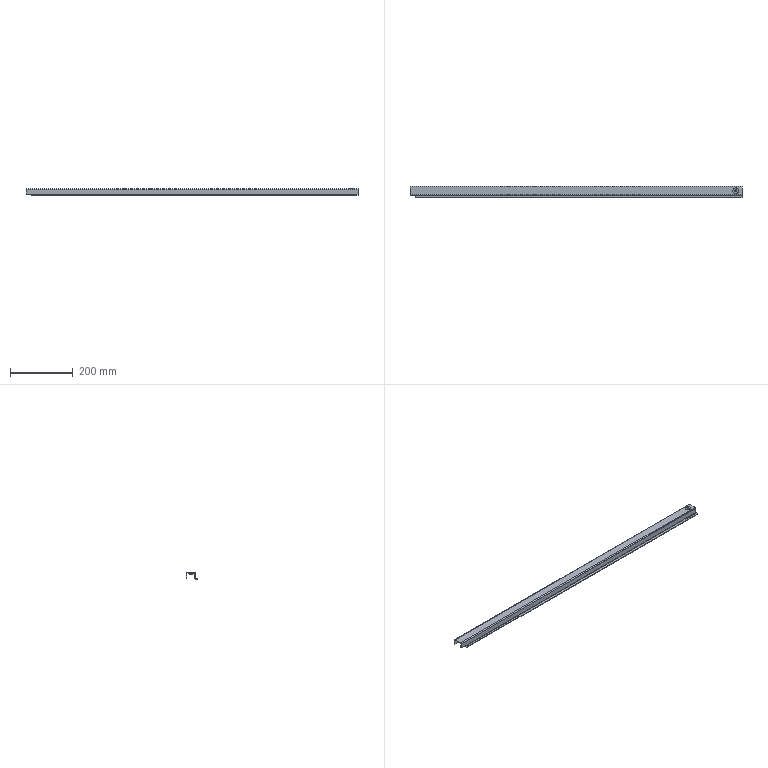Part | SolidWorks | features BaseBody 1 | 1 solid | 48 faces | box 1059 x 38 x 22 mm | volume 155264 mm3 | plane 36 | cylinder 12 | commonest cylinder face diameters 6 x5 2 x3 6.5 x2 18 x2
STEP:
#1=CARTESIAN_POINT('',(500.5,0.,-0.01));
#2=VERTEX_POINT('',#1);
#3=CARTESIAN_POINT('',(500.5,0.,0.));
#4=VERTEX_POINT('',#3);
#5=CARTESIAN_POINT('',(500.5,0.,-0.01));
#6=DIRECTION('',(0.,0.,1.));
#7=VECTOR('',#6,1000.);
#8=LINE('',#5,#7);
#9=EDGE_CURVE('',#2,#4,#8,.T.);
#10=ORIENTED_EDGE('',*,*,#9,.F.);
#11=CARTESIAN_POINT('',(518.5,0.,-0.01));
#12=VERTEX_POINT('',#11);
#13=CARTESIAN_POINT('',(509.5,0.,-0.01));
#14=DIRECTION('',(0.,0.,1.));
#15=DIRECTION('',(1.,0.,0.));
#16=AXIS2_PLACEMENT_3D('',#13,#14,#15);
#17=CIRCLE('',#16,9.);
#18=EDGE_CURVE('',#12,#2,#17,.T.);
#19=ORIENTED_EDGE('',*,*,#18,.F.);
#20=CARTESIAN_POINT('',(518.5,0.,0.));
#21=VERTEX_POINT('',#20);
#22=CARTESIAN_POINT('',(518.5,0.,-0.01));
#23=DIRECTION('',(0.,0.,1.));
#24=VECTOR('',#23,1000.);
#25=LINE('',#22,#24);
#26=EDGE_CURVE('',#12,#21,#25,.T.);
#27=ORIENTED_EDGE('',*,*,#26,.T.);
#28=CARTESIAN_POINT('',(509.5,0.,0.));
#29=DIRECTION('',(0.,0.,1.));
#30=DIRECTION('',(1.,0.,0.));
#31=AXIS2_PLACEMENT_3D('',#28,#29,#30);
#32=CIRCLE('',#31,9.);
#33=EDGE_CURVE('',#21,#4,#32,.T.);
#34=ORIENTED_EDGE('',*,*,#33,.T.);
#35=EDGE_LOOP('',(#10,#19,#27,#34));
#36=FACE_OUTER_BOUND('',#35,.T.);
#37=CARTESIAN_POINT('',(509.5,0.,-0.01));
#38=DIRECTION('',(0.,0.,1.));
#39=DIRECTION('',(1.,0.,0.));
#40=AXIS2_PLACEMENT_3D('',#37,#38,#39);
#41=CYLINDRICAL_SURFACE('',#40,9.);
#42=ADVANCED_FACE('',(#36),#41,.F.);
#43=CARTESIAN_POINT('',(512.75,0.,-0.01));
#44=VERTEX_POINT('',#43);
#45=CARTESIAN_POINT('',(506.25,0.,-0.01));
#46=VERTEX_POINT('',#45);
#47=CARTESIAN_POINT('',(509.5,0.,-0.01));
#48=DIRECTION('',(0.,0.,-1.));
#49=DIRECTION('',(1.,0.,0.));
#50=AXIS2_PLACEMENT_3D('',#47,#48,#49);
#51=CIRCLE('',#50,3.25);
#52=EDGE_CURVE('',#44,#46,#51,.T.);
#53=ORIENTED_EDGE('',*,*,#52,.T.);
#54=CARTESIAN_POINT('',(509.5,0.,-0.01));
#55=DIRECTION('',(0.,0.,-1.));
#56=DIRECTION('',(1.,0.,0.));
#57=AXIS2_PLACEMENT_3D('',#54,#55,#56);
#58=CIRCLE('',#57,3.25);
#59=EDGE_CURVE('',#46,#44,#58,.T.);
#60=ORIENTED_EDGE('',*,*,#59,.T.);
#61=EDGE_LOOP('',(#53,#60));
#62=FACE_BOUND('',#61,.T.);
#63=ORIENTED_EDGE('',*,*,#18,.T.);
#64=CARTESIAN_POINT('',(509.5,0.,-0.01));
#65=DIRECTION('',(0.,0.,1.));
#66=DIRECTION('',(1.,0.,0.));
#67=AXIS2_PLACEMENT_3D('',#64,#65,#66);
#68=CIRCLE('',#67,9.);
#69=EDGE_CURVE('',#2,#12,#68,.T.);
#70=ORIENTED_EDGE('',*,*,#69,.T.);
#71=EDGE_LOOP('',(#63,#70));
#72=FACE_OUTER_BOUND('',#71,.T.);
#73=CARTESIAN_POINT('',(509.5,0.,-0.01));
#74=DIRECTION('',(0.,0.,1.));
#75=DIRECTION('',(1.,0.,0.));
#76=AXIS2_PLACEMENT_3D('',#73,#74,#75);
#77=PLANE('',#76);
#78=ADVANCED_FACE('',(#62,#72),#77,.T.);
#79=CARTESIAN_POINT('',(506.5,0.,-7.));
#80=VERTEX_POINT('',#79);
#81=CARTESIAN_POINT('',(506.5,0.,-2.));
#82=VERTEX_POINT('',#81);
#83=CARTESIAN_POINT('',(506.5,0.,-7.));
#84=DIRECTION('',(0.,0.,1.));
#85=VECTOR('',#84,1000.);
#86=LINE('',#83,#85);
#87=EDGE_CURVE('',#80,#82,#86,.T.);
#88=ORIENTED_EDGE('',*,*,#87,.F.);
#89=CARTESIAN_POINT('',(512.5,0.,-7.));
#90=VERTEX_POINT('',#89);
#91=CARTESIAN_POINT('',(509.5,0.,-7.));
#92=DIRECTION('',(0.,0.,-1.));
#93=DIRECTION('',(-1.,0.,0.));
#94=AXIS2_PLACEMENT_3D('',#91,#92,#93);
#95=CIRCLE('',#94,3.);
#96=EDGE_CURVE('',#80,#90,#95,.T.);
#97=ORIENTED_EDGE('',*,*,#96,.T.);
#98=CARTESIAN_POINT('',(512.5,0.,-2.));
#99=VERTEX_POINT('',#98);
#100=CARTESIAN_POINT('',(512.5,0.,-7.));
#101=DIRECTION('',(0.,0.,1.));
#102=VECTOR('',#101,1000.);
#103=LINE('',#100,#102);
#104=EDGE_CURVE('',#90,#99,#103,.T.);
#105=ORIENTED_EDGE('',*,*,#104,.T.);
#106=CARTESIAN_POINT('',(509.5,0.,-2.));
#107=DIRECTION('',(0.,0.,-1.));
#108=DIRECTION('',(-1.,0.,0.));
#109=AXIS2_PLACEMENT_3D('',#106,#107,#108);
#110=CIRCLE('',#109,3.);
#111=EDGE_CURVE('',#82,#99,#110,.T.);
#112=ORIENTED_EDGE('',*,*,#111,.F.);
#113=EDGE_LOOP('',(#88,#97,#105,#112));
#114=FACE_OUTER_BOUND('',#113,.T.);
#115=CARTESIAN_POINT('',(509.5,0.,-7.));
#116=DIRECTION('',(0.,0.,1.));
#117=DIRECTION('',(1.,0.,0.));
#118=AXIS2_PLACEMENT_3D('',#115,#116,#117);
#119=CYLINDRICAL_SURFACE('',#118,3.);
#120=ADVANCED_FACE('',(#114),#119,.F.);
#121=CARTESIAN_POINT('',(512.387,-5.,-2.));
#122=VERTEX_POINT('',#121);
#123=CARTESIAN_POINT('',(506.613,-5.,-2.));
#124=VERTEX_POINT('',#123);
#125=CARTESIAN_POINT('',(512.387,-5.,-2.));
#126=DIRECTION('',(-1.,0.,0.));
#127=VECTOR('',#126,1000.);
#128=LINE('',#125,#127);
#129=EDGE_CURVE('',#122,#124,#128,.T.);
#130=ORIENTED_EDGE('',*,*,#129,.T.);
#131=CARTESIAN_POINT('',(506.613,-5.,-7.));
#132=VERTEX_POINT('',#131);
#133=CARTESIAN_POINT('',(506.613,-5.,-7.));
#134=DIRECTION('',(0.,0.,1.));
#135=VECTOR('',#134,1000.);
#136=LINE('',#133,#135);
#137=EDGE_CURVE('',#132,#124,#136,.T.);
#138=ORIENTED_EDGE('',*,*,#137,.F.);
#139=CARTESIAN_POINT('',(512.387,-5.,-7.));
#140=VERTEX_POINT('',#139);
#141=CARTESIAN_POINT('',(512.387,-5.,-7.));
#142=DIRECTION('',(-1.,0.,0.));
#143=VECTOR('',#142,1000.);
#144=LINE('',#141,#143);
#145=EDGE_CURVE('',#140,#132,#144,.T.);
#146=ORIENTED_EDGE('',*,*,#145,.F.);
#147=CARTESIAN_POINT('',(512.387,-5.,-7.));
#148=DIRECTION('',(0.,0.,1.));
#149=VECTOR('',#148,1000.);
#150=LINE('',#147,#149);
#151=EDGE_CURVE('',#140,#122,#150,.T.);
#152=ORIENTED_EDGE('',*,*,#151,.T.);
#153=EDGE_LOOP('',(#130,#138,#146,#152));
#154=FACE_OUTER_BOUND('',#153,.T.);
#155=CARTESIAN_POINT('',(512.387,-5.,-7.));
#156=DIRECTION('',(0.,1.,0.));
#157=DIRECTION('',(1.,0.,0.));
#158=AXIS2_PLACEMENT_3D('',#155,#156,#157);
#159=PLANE('',#158);
#160=ADVANCED_FACE('',(#154),#159,.F.);
#161=CARTESIAN_POINT('',(515.274,0.,-2.));
#162=VERTEX_POINT('',#161);
#163=CARTESIAN_POINT('',(515.274,0.,-2.));
#164=DIRECTION('',(-0.5,-0.866,0.));
#165=VECTOR('',#164,1000.);
#166=LINE('',#163,#165);
#167=EDGE_CURVE('',#162,#122,#166,.T.);
#168=ORIENTED_EDGE('',*,*,#167,.T.);
#169=ORIENTED_EDGE('',*,*,#151,.F.);
#170=CARTESIAN_POINT('',(515.274,0.,-7.));
#171=VERTEX_POINT('',#170);
#172=CARTESIAN_POINT('',(515.274,0.,-7.));
#173=DIRECTION('',(-0.5,-0.866,0.));
#174=VECTOR('',#173,1000.);
#175=LINE('',#172,#174);
#176=EDGE_CURVE('',#171,#140,#175,.T.);
#177=ORIENTED_EDGE('',*,*,#176,.F.);
#178=CARTESIAN_POINT('',(515.274,0.,-7.));
#179=DIRECTION('',(0.,0.,1.));
#180=VECTOR('',#179,1000.);
#181=LINE('',#178,#180);
#182=EDGE_CURVE('',#171,#162,#181,.T.);
#183=ORIENTED_EDGE('',*,*,#182,.T.);
#184=EDGE_LOOP('',(#168,#169,#177,#183));
#185=FACE_OUTER_BOUND('',#184,.T.);
#186=CARTESIAN_POINT('',(515.274,0.,-7.));
#187=DIRECTION('',(-0.866,0.5,0.));
#188=DIRECTION('',(0.,0.,1.));
#189=AXIS2_PLACEMENT_3D('',#186,#187,#188);
#190=PLANE('',#189);
#191=ADVANCED_FACE('',(#185),#190,.F.);
#192=CARTESIAN_POINT('',(512.387,5.,-2.));
#193=VERTEX_POINT('',#192);
#194=CARTESIAN_POINT('',(512.387,5.,-2.));
#195=DIRECTION('',(0.5,-0.866,0.));
#196=VECTOR('',#195,1000.);
#197=LINE('',#194,#196);
#198=EDGE_CURVE('',#193,#162,#197,.T.);
#199=ORIENTED_EDGE('',*,*,#198,.T.);
#200=ORIENTED_EDGE('',*,*,#182,.F.);
#201=CARTESIAN_POINT('',(512.387,5.,-7.));
#202=VERTEX_POINT('',#201);
#203=CARTESIAN_POINT('',(512.387,5.,-7.));
#204=DIRECTION('',(0.5,-0.866,0.));
#205=VECTOR('',#204,1000.);
#206=LINE('',#203,#205);
#207=EDGE_CURVE('',#202,#171,#206,.T.);
#208=ORIENTED_EDGE('',*,*,#207,.F.);
#209=CARTESIAN_POINT('',(512.387,5.,-7.));
#210=DIRECTION('',(0.,0.,1.));
#211=VECTOR('',#210,1000.);
#212=LINE('',#209,#211);
#213=EDGE_CURVE('',#202,#193,#212,.T.);
#214=ORIENTED_EDGE('',*,*,#213,.T.);
#215=EDGE_LOOP('',(#199,#200,#208,#214));
#216=FACE_OUTER_BOUND('',#215,.T.);
#217=CARTESIAN_POINT('',(512.387,5.,-7.));
#218=DIRECTION('',(-0.866,-0.5,0.));
#219=DIRECTION('',(-0.5,0.866,0.));
#220=AXIS2_PLACEMENT_3D('',#217,#218,#219);
#221=PLANE('',#220);
#222=ADVANCED_FACE('',(#216),#221,.F.);
#223=CARTESIAN_POINT('',(506.613,5.,-2.));
#224=VERTEX_POINT('',#223);
#225=CARTESIAN_POINT('',(506.613,5.,-2.));
#226=DIRECTION('',(1.,0.,0.));
#227=VECTOR('',#226,1000.);
#228=LINE('',#225,#227);
#229=EDGE_CURVE('',#224,#193,#228,.T.);
#230=ORIENTED_EDGE('',*,*,#229,.T.);
#231=ORIENTED_EDGE('',*,*,#213,.F.);
#232=CARTESIAN_POINT('',(506.613,5.,-7.));
#233=VERTEX_POINT('',#232);
#234=CARTESIAN_POINT('',(506.613,5.,-7.));
#235=DIRECTION('',(1.,0.,0.));
#236=VECTOR('',#235,1000.);
#237=LINE('',#234,#236);
#238=EDGE_CURVE('',#233,#202,#237,.T.);
#239=ORIENTED_EDGE('',*,*,#238,.F.);
#240=CARTESIAN_POINT('',(506.613,5.,-7.));
#241=DIRECTION('',(0.,0.,1.));
#242=VECTOR('',#241,1000.);
#243=LINE('',#240,#242);
#244=EDGE_CURVE('',#233,#224,#243,.T.);
#245=ORIENTED_EDGE('',*,*,#244,.T.);
#246=EDGE_LOOP('',(#230,#231,#239,#245));
#247=FACE_OUTER_BOUND('',#246,.T.);
#248=CARTESIAN_POINT('',(506.613,5.,-7.));
#249=DIRECTION('',(0.,-1.,0.));
#250=DIRECTION('',(0.,0.,-1.));
#251=AXIS2_PLACEMENT_3D('',#248,#249,#250);
#252=PLANE('',#251);
#253=ADVANCED_FACE('',(#247),#252,.F.);
#254=CARTESIAN_POINT('',(503.726,0.,-2.));
#255=VERTEX_POINT('',#254);
#256=CARTESIAN_POINT('',(503.726,0.,-2.));
#257=DIRECTION('',(0.5,0.866,0.));
#258=VECTOR('',#257,1000.);
#259=LINE('',#256,#258);
#260=EDGE_CURVE('',#255,#224,#259,.T.);
#261=ORIENTED_EDGE('',*,*,#260,.T.);
#262=ORIENTED_EDGE('',*,*,#244,.F.);
#263=CARTESIAN_POINT('',(503.726,0.,-7.));
#264=VERTEX_POINT('',#263);
#265=CARTESIAN_POINT('',(503.726,0.,-7.));
#266=DIRECTION('',(0.5,0.866,0.));
#267=VECTOR('',#266,1000.);
#268=LINE('',#265,#267);
#269=EDGE_CURVE('',#264,#233,#268,.T.);
#270=ORIENTED_EDGE('',*,*,#269,.F.);
#271=CARTESIAN_POINT('',(503.726,0.,-7.));
#272=DIRECTION('',(0.,0.,1.));
#273=VECTOR('',#272,1000.);
#274=LINE('',#271,#273);
#275=EDGE_CURVE('',#264,#255,#274,.T.);
#276=ORIENTED_EDGE('',*,*,#275,.T.);
#277=EDGE_LOOP('',(#261,#262,#270,#276));
#278=FACE_OUTER_BOUND('',#277,.T.);
#279=CARTESIAN_POINT('',(503.726,0.,-7.));
#280=DIRECTION('',(0.866,-0.5,0.));
#281=DIRECTION('',(0.,0.,-1.));
#282=AXIS2_PLACEMENT_3D('',#279,#280,#281);
#283=PLANE('',#282);
#284=ADVANCED_FACE('',(#278),#283,.F.);
#285=CARTESIAN_POINT('',(506.613,-5.,-2.));
#286=DIRECTION('',(-0.5,0.866,0.));
#287=VECTOR('',#286,1000.);
#288=LINE('',#285,#287);
#289=EDGE_CURVE('',#124,#255,#288,.T.);
#290=ORIENTED_EDGE('',*,*,#289,.T.);
#291=ORIENTED_EDGE('',*,*,#275,.F.);
#292=CARTESIAN_POINT('',(506.613,-5.,-7.));
#293=DIRECTION('',(-0.5,0.866,0.));
#294=VECTOR('',#293,1000.);
#295=LINE('',#292,#294);
#296=EDGE_CURVE('',#132,#264,#295,.T.);
#297=ORIENTED_EDGE('',*,*,#296,.F.);
#298=ORIENTED_EDGE('',*,*,#137,.T.);
#299=EDGE_LOOP('',(#290,#291,#297,#298));
#300=FACE_OUTER_BOUND('',#299,.T.);
#301=CARTESIAN_POINT('',(506.613,-5.,-7.));
#302=DIRECTION('',(0.866,0.5,0.));
#303=DIRECTION('',(0.,0.,-1.));
#304=AXIS2_PLACEMENT_3D('',#301,#302,#303);
#305=PLANE('',#304);
#306=ADVANCED_FACE('',(#300),#305,.F.);
#307=CARTESIAN_POINT('',(509.5,0.,-7.));
#308=DIRECTION('',(0.,0.,-1.));
#309=DIRECTION('',(-1.,0.,0.));
#310=AXIS2_PLACEMENT_3D('',#307,#308,#309);
#311=CIRCLE('',#310,3.);
#312=EDGE_CURVE('',#90,#80,#311,.T.);
#313=ORIENTED_EDGE('',*,*,#312,.F.);
#314=ORIENTED_EDGE('',*,*,#96,.F.);
#315=EDGE_LOOP('',(#313,#314));
#316=FACE_BOUND('',#315,.T.);
#317=ORIENTED_EDGE('',*,*,#296,.T.);
#318=ORIENTED_EDGE('',*,*,#269,.T.);
#319=ORIENTED_EDGE('',*,*,#238,.T.);
#320=ORIENTED_EDGE('',*,*,#207,.T.);
#321=ORIENTED_EDGE('',*,*,#176,.T.);
#322=ORIENTED_EDGE('',*,*,#145,.T.);
#323=EDGE_LOOP('',(#317,#318,#319,#320,#321,#322));
#324=FACE_OUTER_BOUND('',#323,.T.);
#325=CARTESIAN_POINT('',(0.,0.,-7.));
#326=DIRECTION('',(0.,0.,-1.));
#327=DIRECTION('',(0.,-1.,0.));
#328=AXIS2_PLACEMENT_3D('',#325,#326,#327);
#329=PLANE('',#328);
#330=ADVANCED_FACE('',(#316,#324),#329,.T.);
#331=CARTESIAN_POINT('',(509.5,0.,-2.));
#332=DIRECTION('',(0.,0.,-1.));
#333=DIRECTION('',(-1.,0.,0.));
#334=AXIS2_PLACEMENT_3D('',#331,#332,#333);
#335=CIRCLE('',#334,3.);
#336=EDGE_CURVE('',#99,#82,#335,.T.);
#337=ORIENTED_EDGE('',*,*,#336,.T.);
#338=ORIENTED_EDGE('',*,*,#111,.T.);
#339=EDGE_LOOP('',(#337,#338));
#340=FACE_BOUND('',#339,.T.);
#341=CARTESIAN_POINT('',(512.75,0.,-2.));
#342=VERTEX_POINT('',#341);
#343=CARTESIAN_POINT('',(506.25,0.,-2.));
#344=VERTEX_POINT('',#343);
#345=CARTESIAN_POINT('',(509.5,0.,-2.));
#346=DIRECTION('',(0.,0.,1.));
#347=DIRECTION('',(1.,0.,0.));
#348=AXIS2_PLACEMENT_3D('',#345,#346,#347);
#349=CIRCLE('',#348,3.25);
#350=EDGE_CURVE('',#342,#344,#349,.T.);
#351=ORIENTED_EDGE('',*,*,#350,.T.);
#352=CARTESIAN_POINT('',(509.5,0.,-2.));
#353=DIRECTION('',(0.,0.,1.));
#354=DIRECTION('',(1.,0.,0.));
#355=AXIS2_PLACEMENT_3D('',#352,#353,#354);
#356=CIRCLE('',#355,3.25);
#357=EDGE_CURVE('',#344,#342,#356,.T.);
#358=ORIENTED_EDGE('',*,*,#357,.T.);
#359=EDGE_LOOP('',(#351,#358));
#360=FACE_OUTER_BOUND('',#359,.T.);
#361=CARTESIAN_POINT('',(0.,0.,-2.));
#362=DIRECTION('',(0.,0.,-1.));
#363=DIRECTION('',(0.,-1.,0.));
#364=AXIS2_PLACEMENT_3D('',#361,#362,#363);
#365=PLANE('',#364);
#366=ADVANCED_FACE('',(#340,#360),#365,.F.);
#367=CARTESIAN_POINT('',(-511.5,13.,-18.));
#368=VERTEX_POINT('',#367);
#369=CARTESIAN_POINT('',(-511.5,15.,-18.));
#370=VERTEX_POINT('',#369);
#371=CARTESIAN_POINT('',(-511.5,-23.,-18.));
#372=DIRECTION('',(0.,1.,0.));
#373=VECTOR('',#372,1000.);
#374=LINE('',#371,#373);
#375=EDGE_CURVE('',#368,#370,#374,.T.);
#376=ORIENTED_EDGE('',*,*,#375,.T.);
#377=CARTESIAN_POINT('',(-511.5,15.,-20.));
#378=VERTEX_POINT('',#377);
#379=CARTESIAN_POINT('',(-511.5,15.,-20.));
#380=DIRECTION('',(0.,0.,-1.));
#381=VECTOR('',#380,1000.);
#382=LINE('',#379,#381);
#383=EDGE_CURVE('',#370,#378,#382,.T.);
#384=ORIENTED_EDGE('',*,*,#383,.T.);
#385=CARTESIAN_POINT('',(-511.5,13.,-20.));
#386=VERTEX_POINT('',#385);
#387=CARTESIAN_POINT('',(-511.5,-23.,-20.));
#388=DIRECTION('',(0.,1.,0.));
#389=VECTOR('',#388,1000.);
#390=LINE('',#387,#389);
#391=EDGE_CURVE('',#386,#378,#390,.T.);
#392=ORIENTED_EDGE('',*,*,#391,.F.);
#393=CARTESIAN_POINT('',(-511.5,13.,0.));
#394=DIRECTION('',(0.,0.,-1.));
#395=VECTOR('',#394,1000.);
#396=LINE('',#393,#395);
#397=EDGE_CURVE('',#368,#386,#396,.T.);
#398=ORIENTED_EDGE('',*,*,#397,.F.);
#399=EDGE_LOOP('',(#376,#384,#392,#398));
#400=FACE_OUTER_BOUND('',#399,.T.);
#401=CARTESIAN_POINT('',(-511.5,-23.,-20.));
#402=DIRECTION('',(1.,0.,0.));
#403=DIRECTION('',(0.,1.,0.));
#404=AXIS2_PLACEMENT_3D('',#401,#402,#403);
#405=PLANE('',#404);
#406=ADVANCED_FACE('',(#400),#405,.F.);
#407=CARTESIAN_POINT('',(-529.5,13.,-18.));
#408=VERTEX_POINT('',#407);
#409=CARTESIAN_POINT('',(-529.5,15.,-18.));
#410=VERTEX_POINT('',#409);
#411=CARTESIAN_POINT('',(-529.5,-23.,-18.));
#412=DIRECTION('',(0.,1.,0.));
#413=VECTOR('',#412,1000.);
#414=LINE('',#411,#413);
#415=EDGE_CURVE('',#408,#410,#414,.T.);
#416=ORIENTED_EDGE('',*,*,#415,.T.);
#417=CARTESIAN_POINT('',(-529.5,15.,-18.));
#418=DIRECTION('',(1.,0.,0.));
#419=VECTOR('',#418,1000.);
#420=LINE('',#417,#419);
#421=EDGE_CURVE('',#410,#370,#420,.T.);
#422=ORIENTED_EDGE('',*,*,#421,.T.);
#423=ORIENTED_EDGE('',*,*,#375,.F.);
#424=CARTESIAN_POINT('',(0.,13.,-18.));
#425=DIRECTION('',(1.,0.,0.));
#426=VECTOR('',#425,1000.);
#427=LINE('',#424,#426);
#428=EDGE_CURVE('',#408,#368,#427,.T.);
#429=ORIENTED_EDGE('',*,*,#428,.F.);
#430=EDGE_LOOP('',(#416,#422,#423,#429));
#431=FACE_OUTER_BOUND('',#430,.T.);
#432=CARTESIAN_POINT('',(-529.5,-23.,-18.));
#433=DIRECTION('',(0.,0.,1.));
#434=DIRECTION('',(0.,-1.,0.));
#435=AXIS2_PLACEMENT_3D('',#432,#433,#434);
#436=PLANE('',#435);
#437=ADVANCED_FACE('',(#431),#436,.F.);
#438=CARTESIAN_POINT('',(529.5,-23.,-20.));
#439=VERTEX_POINT('',#438);
#440=CARTESIAN_POINT('',(-511.5,-23.,-20.));
#441=VERTEX_POINT('',#440);
#442=CARTESIAN_POINT('',(-511.5,-23.,-20.));
#443=DIRECTION('',(-1.,0.,0.));
#444=VECTOR('',#443,1000.);
#445=LINE('',#442,#444);
#446=EDGE_CURVE('',#439,#441,#445,.T.);
#447=ORIENTED_EDGE('',*,*,#446,.T.);
#448=CARTESIAN_POINT('',(-511.5,-23.,-22.));
#449=VERTEX_POINT('',#448);
#450=CARTESIAN_POINT('',(-511.5,-23.,-22.));
#451=DIRECTION('',(0.,0.,1.));
#452=VECTOR('',#451,1000.);
#453=LINE('',#450,#452);
#454=EDGE_CURVE('',#449,#441,#453,.T.);
#455=ORIENTED_EDGE('',*,*,#454,.F.);
#456=CARTESIAN_POINT('',(529.5,-23.,-22.));
#457=VERTEX_POINT('',#456);
#458=CARTESIAN_POINT('',(-511.5,-23.,-22.));
#459=DIRECTION('',(-1.,0.,0.));
#460=VECTOR('',#459,1000.);
#461=LINE('',#458,#460);
#462=EDGE_CURVE('',#457,#449,#461,.T.);
#463=ORIENTED_EDGE('',*,*,#462,.F.);
#464=CARTESIAN_POINT('',(529.5,-23.,-22.));
#465=DIRECTION('',(0.,0.,1.));
#466=VECTOR('',#465,1000.);
#467=LINE('',#464,#466);
#468=EDGE_CURVE('',#457,#439,#467,.T.);
#469=ORIENTED_EDGE('',*,*,#468,.T.);
#470=EDGE_LOOP('',(#447,#455,#463,#469));
#471=FACE_OUTER_BOUND('',#470,.T.);
#472=CARTESIAN_POINT('',(-511.5,-23.,-22.));
#473=DIRECTION('',(0.,1.,0.));
#474=DIRECTION('',(0.,0.,-1.));
#475=AXIS2_PLACEMENT_3D('',#472,#473,#474);
#476=PLANE('',#475);
#477=ADVANCED_FACE('',(#471),#476,.F.);
#478=CARTESIAN_POINT('',(529.5,-16.,-20.));
#479=VERTEX_POINT('',#478);
#480=CARTESIAN_POINT('',(529.5,-23.,-20.));
#481=DIRECTION('',(0.,-1.,0.));
#482=VECTOR('',#481,1000.);
#483=LINE('',#480,#482);
#484=EDGE_CURVE('',#479,#439,#483,.T.);
#485=ORIENTED_EDGE('',*,*,#484,.F.);
#486=CARTESIAN_POINT('',(-511.5,-16.,-20.));
#487=VERTEX_POINT('',#486);
#488=CARTESIAN_POINT('',(-511.5,-16.,-20.));
#489=DIRECTION('',(1.,0.,0.));
#490=VECTOR('',#489,1000.);
#491=LINE('',#488,#490);
#492=EDGE_CURVE('',#487,#479,#491,.T.);
#493=ORIENTED_EDGE('',*,*,#492,.F.);
#494=CARTESIAN_POINT('',(-511.5,-15.,-20.));
#495=DIRECTION('',(0.,1.,0.));
#496=VECTOR('',#495,1000.);
#497=LINE('',#494,#496);
#498=EDGE_CURVE('',#441,#487,#497,.T.);
#499=ORIENTED_EDGE('',*,*,#498,.F.);
#500=ORIENTED_EDGE('',*,*,#446,.F.);
#501=EDGE_LOOP('',(#485,#493,#499,#500));
#502=FACE_OUTER_BOUND('',#501,.T.);
#503=CARTESIAN_POINT('',(0.,0.,-20.));
#504=DIRECTION('',(0.,0.,1.));
#505=DIRECTION('',(1.,0.,0.));
#506=AXIS2_PLACEMENT_3D('',#503,#504,#505);
#507=PLANE('',#506);
#508=ADVANCED_FACE('',(#502),#507,.T.);
#509=CARTESIAN_POINT('',(529.5,-16.,-22.));
#510=VERTEX_POINT('',#509);
#511=CARTESIAN_POINT('',(-511.5,-16.,-22.));
#512=VERTEX_POINT('',#511);
#513=CARTESIAN_POINT('',(0.,-16.,-22.));
#514=DIRECTION('',(-1.,0.,0.));
#515=VECTOR('',#514,1000.);
#516=LINE('',#513,#515);
#517=EDGE_CURVE('',#510,#512,#516,.T.);
#518=ORIENTED_EDGE('',*,*,#517,.F.);
#519=CARTESIAN_POINT('',(529.5,-23.,-22.));
#520=DIRECTION('',(0.,-1.,0.));
#521=VECTOR('',#520,1000.);
#522=LINE('',#519,#521);
#523=EDGE_CURVE('',#510,#457,#522,.T.);
#524=ORIENTED_EDGE('',*,*,#523,.T.);
#525=ORIENTED_EDGE('',*,*,#462,.T.);
#526=CARTESIAN_POINT('',(-511.5,-15.,-22.));
#527=DIRECTION('',(0.,1.,0.));
#528=VECTOR('',#527,1000.);
#529=LINE('',#526,#528);
#530=EDGE_CURVE('',#449,#512,#529,.T.);
#531=ORIENTED_EDGE('',*,*,#530,.T.);
#532=EDGE_LOOP('',(#518,#524,#525,#531));
#533=FACE_OUTER_BOUND('',#532,.T.);
#534=CARTESIAN_POINT('',(0.,0.,-22.));
#535=DIRECTION('',(0.,0.,1.));
#536=DIRECTION('',(1.,0.,0.));
#537=AXIS2_PLACEMENT_3D('',#534,#535,#536);
#538=PLANE('',#537);
#539=ADVANCED_FACE('',(#533),#538,.F.);
#540=CARTESIAN_POINT('',(-511.5,-16.,-20.));
#541=DIRECTION('',(0.,0.,-1.));
#542=VECTOR('',#541,1000.);
#543=LINE('',#540,#542);
#544=EDGE_CURVE('',#487,#512,#543,.T.);
#545=ORIENTED_EDGE('',*,*,#544,.T.);
#546=ORIENTED_EDGE('',*,*,#530,.F.);
#547=ORIENTED_EDGE('',*,*,#454,.T.);
#548=ORIENTED_EDGE('',*,*,#498,.T.);
#549=EDGE_LOOP('',(#545,#546,#547,#548));
#550=FACE_OUTER_BOUND('',#549,.T.);
#551=CARTESIAN_POINT('',(-511.5,-15.,-22.));
#552=DIRECTION('',(1.,0.,0.));
#553=DIRECTION('',(0.,0.,-1.));
#554=AXIS2_PLACEMENT_3D('',#551,#552,#553);
#555=PLANE('',#554);
#556=ADVANCED_FACE('',(#550),#555,.F.);
#557=CARTESIAN_POINT('',(529.5,-16.,-20.));
#558=DIRECTION('',(0.,0.,-1.));
#559=VECTOR('',#558,1000.);
#560=LINE('',#557,#559);
#561=EDGE_CURVE('',#479,#510,#560,.T.);
#562=ORIENTED_EDGE('',*,*,#561,.F.);
#563=ORIENTED_EDGE('',*,*,#484,.T.);
#564=ORIENTED_EDGE('',*,*,#468,.F.);
#565=ORIENTED_EDGE('',*,*,#523,.F.);
#566=EDGE_LOOP('',(#562,#563,#564,#565));
#567=FACE_OUTER_BOUND('',#566,.T.);
#568=CARTESIAN_POINT('',(529.5,-23.,-22.));
#569=DIRECTION('',(-1.,0.,0.));
#570=DIRECTION('',(0.,1.,0.));
#571=AXIS2_PLACEMENT_3D('',#568,#569,#570);
#572=PLANE('',#571);
#573=ADVANCED_FACE('',(#567),#572,.F.);
#574=CARTESIAN_POINT('',(529.5,-15.,-19.));
#575=VERTEX_POINT('',#574);
#576=CARTESIAN_POINT('',(-511.5,-15.,-19.));
#577=VERTEX_POINT('',#576);
#578=CARTESIAN_POINT('',(529.5,-15.,-19.));
#579=DIRECTION('',(-1.,0.,0.));
#580=VECTOR('',#579,1000.);
#581=LINE('',#578,#580);
#582=EDGE_CURVE('',#575,#577,#581,.T.);
#583=ORIENTED_EDGE('',*,*,#582,.T.);
#584=CARTESIAN_POINT('',(-511.5,-16.,-19.));
#585=DIRECTION('',(-1.,0.,0.));
#586=DIRECTION('',(0.,0.,-1.));
#587=AXIS2_PLACEMENT_3D('',#584,#585,#586);
#588=CIRCLE('',#587,1.);
#589=EDGE_CURVE('',#577,#487,#588,.T.);
#590=ORIENTED_EDGE('',*,*,#589,.T.);
#591=ORIENTED_EDGE('',*,*,#492,.T.);
#592=CARTESIAN_POINT('',(529.5,-16.,-19.));
#593=DIRECTION('',(1.,0.,0.));
#594=DIRECTION('',(0.,0.,-1.));
#595=AXIS2_PLACEMENT_3D('',#592,#593,#594);
#596=CIRCLE('',#595,1.);
#597=EDGE_CURVE('',#479,#575,#596,.T.);
#598=ORIENTED_EDGE('',*,*,#597,.T.);
#599=EDGE_LOOP('',(#583,#590,#591,#598));
#600=FACE_OUTER_BOUND('',#599,.T.);
#601=CARTESIAN_POINT('',(529.5,-16.,-19.));
#602=DIRECTION('',(1.,0.,0.));
#603=DIRECTION('',(0.,0.,-1.));
#604=AXIS2_PLACEMENT_3D('',#601,#602,#603);
#605=CYLINDRICAL_SURFACE('',#604,1.);
#606=ADVANCED_FACE('',(#600),#605,.F.);
#607=CARTESIAN_POINT('',(529.5,-13.,-19.));
#608=VERTEX_POINT('',#607);
#609=CARTESIAN_POINT('',(-511.5,-13.,-19.));
#610=VERTEX_POINT('',#609);
#611=CARTESIAN_POINT('',(529.5,-13.,-19.));
#612=DIRECTION('',(-1.,0.,0.));
#613=VECTOR('',#612,1000.);
#614=LINE('',#611,#613);
#615=EDGE_CURVE('',#608,#610,#614,.T.);
#616=ORIENTED_EDGE('',*,*,#615,.F.);
#617=CARTESIAN_POINT('',(529.5,-16.,-19.));
#618=DIRECTION('',(1.,0.,0.));
#619=DIRECTION('',(0.,0.,-1.));
#620=AXIS2_PLACEMENT_3D('',#617,#618,#619);
#621=CIRCLE('',#620,3.);
#622=EDGE_CURVE('',#510,#608,#621,.T.);
#623=ORIENTED_EDGE('',*,*,#622,.F.);
#624=ORIENTED_EDGE('',*,*,#517,.T.);
#625=CARTESIAN_POINT('',(-511.5,-16.,-19.));
#626=DIRECTION('',(-1.,0.,0.));
#627=DIRECTION('',(0.,0.,-1.));
#628=AXIS2_PLACEMENT_3D('',#625,#626,#627);
#629=CIRCLE('',#628,3.);
#630=EDGE_CURVE('',#610,#512,#629,.T.);
#631=ORIENTED_EDGE('',*,*,#630,.F.);
#632=EDGE_LOOP('',(#616,#623,#624,#631));
#633=FACE_OUTER_BOUND('',#632,.T.);
#634=CARTESIAN_POINT('',(529.5,-16.,-19.));
#635=DIRECTION('',(1.,0.,0.));
#636=DIRECTION('',(0.,0.,-1.));
#637=AXIS2_PLACEMENT_3D('',#634,#635,#636);
#638=CYLINDRICAL_SURFACE('',#637,3.);
#639=ADVANCED_FACE('',(#633),#638,.T.);
#640=ORIENTED_EDGE('',*,*,#597,.F.);
#641=ORIENTED_EDGE('',*,*,#561,.T.);
#642=ORIENTED_EDGE('',*,*,#622,.T.);
#643=CARTESIAN_POINT('',(529.5,-15.,-19.));
#644=DIRECTION('',(0.,1.,0.));
#645=VECTOR('',#644,1000.);
#646=LINE('',#643,#645);
#647=EDGE_CURVE('',#575,#608,#646,.T.);
#648=ORIENTED_EDGE('',*,*,#647,.F.);
#649=EDGE_LOOP('',(#640,#641,#642,#648));
#650=FACE_OUTER_BOUND('',#649,.T.);
#651=CARTESIAN_POINT('',(529.5,-16.,-19.));
#652=DIRECTION('',(-1.,0.,0.));
#653=DIRECTION('',(0.,0.,1.));
#654=AXIS2_PLACEMENT_3D('',#651,#652,#653);
#655=PLANE('',#654);
#656=ADVANCED_FACE('',(#650),#655,.F.);
#657=CARTESIAN_POINT('',(-511.5,-13.,-18.));
#658=VERTEX_POINT('',#657);
#659=CARTESIAN_POINT('',(-529.5,-13.,-18.));
#660=VERTEX_POINT('',#659);
#661=CARTESIAN_POINT('',(0.,-13.,-18.));
#662=DIRECTION('',(-1.,0.,0.));
#663=VECTOR('',#662,1000.);
#664=LINE('',#661,#663);
#665=EDGE_CURVE('',#658,#660,#664,.T.);
#666=ORIENTED_EDGE('',*,*,#665,.F.);
#667=CARTESIAN_POINT('',(-511.5,-15.,-18.));
#668=VERTEX_POINT('',#667);
#669=CARTESIAN_POINT('',(-511.5,-15.,-18.));
#670=DIRECTION('',(0.,1.,0.));
#671=VECTOR('',#670,1000.);
#672=LINE('',#669,#671);
#673=EDGE_CURVE('',#668,#658,#672,.T.);
#674=ORIENTED_EDGE('',*,*,#673,.F.);
#675=CARTESIAN_POINT('',(-529.5,-15.,-18.));
#676=VERTEX_POINT('',#675);
#677=CARTESIAN_POINT('',(-511.5,-15.,-18.));
#678=DIRECTION('',(-1.,0.,0.));
#679=VECTOR('',#678,1000.);
#680=LINE('',#677,#679);
#681=EDGE_CURVE('',#668,#676,#680,.T.);
#682=ORIENTED_EDGE('',*,*,#681,.T.);
#683=CARTESIAN_POINT('',(-529.5,-23.,-18.));
#684=DIRECTION('',(0.,1.,0.));
#685=VECTOR('',#684,1000.);
#686=LINE('',#683,#685);
#687=EDGE_CURVE('',#676,#660,#686,.T.);
#688=ORIENTED_EDGE('',*,*,#687,.T.);
#689=EDGE_LOOP('',(#666,#674,#682,#688));
#690=FACE_OUTER_BOUND('',#689,.T.);
#691=CARTESIAN_POINT('',(-511.5,-15.,-18.));
#692=DIRECTION('',(0.,0.,-1.));
#693=DIRECTION('',(0.,-1.,0.));
#694=AXIS2_PLACEMENT_3D('',#691,#692,#693);
#695=PLANE('',#694);
#696=ADVANCED_FACE('',(#690),#695,.T.);
#697=CARTESIAN_POINT('',(-511.5,-13.,0.));
#698=DIRECTION('',(0.,0.,1.));
#699=VECTOR('',#698,1000.);
#700=LINE('',#697,#699);
#701=EDGE_CURVE('',#610,#658,#700,.T.);
#702=ORIENTED_EDGE('',*,*,#701,.F.);
#703=ORIENTED_EDGE('',*,*,#630,.T.);
#704=ORIENTED_EDGE('',*,*,#544,.F.);
#705=ORIENTED_EDGE('',*,*,#589,.F.);
#706=CARTESIAN_POINT('',(-511.5,-15.,-19.));
#707=DIRECTION('',(0.,0.,1.));
#708=VECTOR('',#707,1000.);
#709=LINE('',#706,#708);
#710=EDGE_CURVE('',#577,#668,#709,.T.);
#711=ORIENTED_EDGE('',*,*,#710,.T.);
#712=ORIENTED_EDGE('',*,*,#673,.T.);
#713=EDGE_LOOP('',(#702,#703,#704,#705,#711,#712));
#714=FACE_OUTER_BOUND('',#713,.T.);
#715=CARTESIAN_POINT('',(-511.5,-15.,-19.));
#716=DIRECTION('',(-1.,0.,0.));
#717=DIRECTION('',(0.,1.,0.));
#718=AXIS2_PLACEMENT_3D('',#715,#716,#717);
#719=PLANE('',#718);
#720=ADVANCED_FACE('',(#714),#719,.T.);
#721=ORIENTED_EDGE('',*,*,#687,.F.);
#722=CARTESIAN_POINT('',(-529.5,-15.,-3.));
#723=VERTEX_POINT('',#722);
#724=CARTESIAN_POINT('',(-529.5,-15.,-20.));
#725=DIRECTION('',(0.,0.,1.));
#726=VECTOR('',#725,1000.);
#727=LINE('',#724,#726);
#728=EDGE_CURVE('',#676,#723,#727,.T.);
#729=ORIENTED_EDGE('',*,*,#728,.T.);
#730=CARTESIAN_POINT('',(-529.5,-13.,-3.));
#731=VERTEX_POINT('',#730);
#732=CARTESIAN_POINT('',(-529.5,-13.,-3.));
#733=DIRECTION('',(0.,-1.,0.));
#734=VECTOR('',#733,1000.);
#735=LINE('',#732,#734);
#736=EDGE_CURVE('',#731,#723,#735,.T.);
#737=ORIENTED_EDGE('',*,*,#736,.F.);
#738=CARTESIAN_POINT('',(-529.5,-13.,0.));
#739=DIRECTION('',(0.,0.,1.));
#740=VECTOR('',#739,1000.);
#741=LINE('',#738,#740);
#742=EDGE_CURVE('',#660,#731,#741,.T.);
#743=ORIENTED_EDGE('',*,*,#742,.F.);
#744=EDGE_LOOP('',(#721,#729,#737,#743));
#745=FACE_OUTER_BOUND('',#744,.T.);
#746=CARTESIAN_POINT('',(-529.5,-15.,-20.));
#747=DIRECTION('',(-1.,0.,0.));
#748=DIRECTION('',(0.,0.,1.));
#749=AXIS2_PLACEMENT_3D('',#746,#747,#748);
#750=PLANE('',#749);
#751=ADVANCED_FACE('',(#745),#750,.T.);
#752=CARTESIAN_POINT('',(-529.5,-12.,-2.));
#753=VERTEX_POINT('',#752);
#754=CARTESIAN_POINT('',(529.5,-12.,-2.));
#755=VERTEX_POINT('',#754);
#756=CARTESIAN_POINT('',(-529.5,-12.,-2.));
#757=DIRECTION('',(1.,0.,0.));
#758=VECTOR('',#757,1000.);
#759=LINE('',#756,#758);
#760=EDGE_CURVE('',#753,#755,#759,.T.);
#761=ORIENTED_EDGE('',*,*,#760,.T.);
#762=CARTESIAN_POINT('',(529.5,-13.,-3.));
#763=VERTEX_POINT('',#762);
#764=CARTESIAN_POINT('',(529.5,-12.,-3.));
#765=DIRECTION('',(1.,0.,0.));
#766=DIRECTION('',(0.,0.,1.));
#767=AXIS2_PLACEMENT_3D('',#764,#765,#766);
#768=CIRCLE('',#767,1.);
#769=EDGE_CURVE('',#755,#763,#768,.T.);
#770=ORIENTED_EDGE('',*,*,#769,.T.);
#771=CARTESIAN_POINT('',(529.5,-13.,-3.));
#772=DIRECTION('',(-1.,0.,0.));
#773=VECTOR('',#772,1000.);
#774=LINE('',#771,#773);
#775=EDGE_CURVE('',#763,#731,#774,.T.);
#776=ORIENTED_EDGE('',*,*,#775,.T.);
#777=CARTESIAN_POINT('',(-529.5,-12.,-3.));
#778=DIRECTION('',(-1.,0.,0.));
#779=DIRECTION('',(0.,0.,1.));
#780=AXIS2_PLACEMENT_3D('',#777,#778,#779);
#781=CIRCLE('',#780,1.);
#782=EDGE_CURVE('',#731,#753,#781,.T.);
#783=ORIENTED_EDGE('',*,*,#782,.T.);
#784=EDGE_LOOP('',(#761,#770,#776,#783));
#785=FACE_OUTER_BOUND('',#784,.T.);
#786=CARTESIAN_POINT('',(-529.5,-12.,-3.));
#787=DIRECTION('',(-1.,0.,0.));
#788=DIRECTION('',(0.,-1.,0.));
#789=AXIS2_PLACEMENT_3D('',#786,#787,#788);
#790=CYLINDRICAL_SURFACE('',#789,1.);
#791=ADVANCED_FACE('',(#785),#790,.F.);
#792=CARTESIAN_POINT('',(-529.5,-12.,0.));
#793=VERTEX_POINT('',#792);
#794=CARTESIAN_POINT('',(529.5,-12.,0.));
#795=VERTEX_POINT('',#794);
#796=CARTESIAN_POINT('',(-529.5,-12.,0.));
#797=DIRECTION('',(1.,0.,0.));
#798=VECTOR('',#797,1000.);
#799=LINE('',#796,#798);
#800=EDGE_CURVE('',#793,#795,#799,.T.);
#801=ORIENTED_EDGE('',*,*,#800,.F.);
#802=CARTESIAN_POINT('',(-529.5,-12.,-3.));
#803=DIRECTION('',(-1.,0.,0.));
#804=DIRECTION('',(0.,0.,1.));
#805=AXIS2_PLACEMENT_3D('',#802,#803,#804);
#806=CIRCLE('',#805,3.);
#807=EDGE_CURVE('',#723,#793,#806,.T.);
#808=ORIENTED_EDGE('',*,*,#807,.F.);
#809=CARTESIAN_POINT('',(529.5,-15.,-3.));
#810=VERTEX_POINT('',#809);
#811=CARTESIAN_POINT('',(529.5,-15.,-3.));
#812=DIRECTION('',(1.,0.,0.));
#813=VECTOR('',#812,1000.);
#814=LINE('',#811,#813);
#815=EDGE_CURVE('',#723,#810,#814,.T.);
#816=ORIENTED_EDGE('',*,*,#815,.T.);
#817=CARTESIAN_POINT('',(529.5,-12.,-3.));
#818=DIRECTION('',(1.,0.,0.));
#819=DIRECTION('',(0.,0.,1.));
#820=AXIS2_PLACEMENT_3D('',#817,#818,#819);
#821=CIRCLE('',#820,3.);
#822=EDGE_CURVE('',#795,#810,#821,.T.);
#823=ORIENTED_EDGE('',*,*,#822,.F.);
#824=EDGE_LOOP('',(#801,#808,#816,#823));
#825=FACE_OUTER_BOUND('',#824,.T.);
#826=CARTESIAN_POINT('',(-529.5,-12.,-3.));
#827=DIRECTION('',(-1.,0.,0.));
#828=DIRECTION('',(0.,-1.,0.));
#829=AXIS2_PLACEMENT_3D('',#826,#827,#828);
#830=CYLINDRICAL_SURFACE('',#829,3.);
#831=ADVANCED_FACE('',(#825),#830,.T.);
#832=ORIENTED_EDGE('',*,*,#782,.F.);
#833=ORIENTED_EDGE('',*,*,#736,.T.);
#834=ORIENTED_EDGE('',*,*,#807,.T.);
#835=CARTESIAN_POINT('',(-529.5,-12.,-2.));
#836=DIRECTION('',(0.,0.,1.));
#837=VECTOR('',#836,1000.);
#838=LINE('',#835,#837);
#839=EDGE_CURVE('',#753,#793,#838,.T.);
#840=ORIENTED_EDGE('',*,*,#839,.F.);
#841=EDGE_LOOP('',(#832,#833,#834,#840));
#842=FACE_OUTER_BOUND('',#841,.T.);
#843=CARTESIAN_POINT('',(-529.5,-12.,-3.));
#844=DIRECTION('',(1.,0.,0.));
#845=DIRECTION('',(0.,1.,0.));
#846=AXIS2_PLACEMENT_3D('',#843,#844,#845);
#847=PLANE('',#846);
#848=ADVANCED_FACE('',(#842),#847,.F.);
#849=CARTESIAN_POINT('',(529.5,-15.,-3.));
#850=DIRECTION('',(0.,-1.,0.));
#851=VECTOR('',#850,1000.);
#852=LINE('',#849,#851);
#853=EDGE_CURVE('',#763,#810,#852,.T.);
#854=ORIENTED_EDGE('',*,*,#853,.F.);
#855=ORIENTED_EDGE('',*,*,#769,.F.);
#856=CARTESIAN_POINT('',(529.5,-12.,-2.));
#857=DIRECTION('',(0.,0.,1.));
#858=VECTOR('',#857,1000.);
#859=LINE('',#856,#858);
#860=EDGE_CURVE('',#755,#795,#859,.T.);
#861=ORIENTED_EDGE('',*,*,#860,.T.);
#862=ORIENTED_EDGE('',*,*,#822,.T.);
#863=EDGE_LOOP('',(#854,#855,#861,#862));
#864=FACE_OUTER_BOUND('',#863,.T.);
#865=CARTESIAN_POINT('',(529.5,-12.,-3.));
#866=DIRECTION('',(1.,0.,0.));
#867=DIRECTION('',(0.,1.,0.));
#868=AXIS2_PLACEMENT_3D('',#865,#866,#867);
#869=PLANE('',#868);
#870=ADVANCED_FACE('',(#864),#869,.T.);
#871=ORIENTED_EDGE('',*,*,#391,.T.);
#872=CARTESIAN_POINT('',(529.5,15.,-20.));
#873=VERTEX_POINT('',#872);
#874=CARTESIAN_POINT('',(529.5,15.,-20.));
#875=DIRECTION('',(1.,0.,0.));
#876=VECTOR('',#875,1000.);
#877=LINE('',#874,#876);
#878=EDGE_CURVE('',#378,#873,#877,.T.);
#879=ORIENTED_EDGE('',*,*,#878,.T.);
#880=CARTESIAN_POINT('',(529.5,13.,-20.));
#881=VERTEX_POINT('',#880);
#882=CARTESIAN_POINT('',(529.5,15.,-20.));
#883=DIRECTION('',(0.,-1.,0.));
#884=VECTOR('',#883,1000.);
#885=LINE('',#882,#884);
#886=EDGE_CURVE('',#873,#881,#885,.T.);
#887=ORIENTED_EDGE('',*,*,#886,.T.);
#888=CARTESIAN_POINT('',(0.,13.,-20.));
#889=DIRECTION('',(1.,0.,0.));
#890=VECTOR('',#889,1000.);
#891=LINE('',#888,#890);
#892=EDGE_CURVE('',#386,#881,#891,.T.);
#893=ORIENTED_EDGE('',*,*,#892,.F.);
#894=EDGE_LOOP('',(#871,#879,#887,#893));
#895=FACE_OUTER_BOUND('',#894,.T.);
#896=CARTESIAN_POINT('',(529.5,15.,-20.));
#897=DIRECTION('',(0.,0.,-1.));
#898=DIRECTION('',(-1.,0.,0.));
#899=AXIS2_PLACEMENT_3D('',#896,#897,#898);
#900=PLANE('',#899);
#901=ADVANCED_FACE('',(#895),#900,.T.);
#902=ORIENTED_EDGE('',*,*,#428,.T.);
#903=ORIENTED_EDGE('',*,*,#397,.T.);
#904=ORIENTED_EDGE('',*,*,#892,.T.);
#905=CARTESIAN_POINT('',(529.5,13.,-3.));
#906=VERTEX_POINT('',#905);
#907=CARTESIAN_POINT('',(529.5,13.,0.));
#908=DIRECTION('',(0.,0.,1.));
#909=VECTOR('',#908,1000.);
#910=LINE('',#907,#909);
#911=EDGE_CURVE('',#881,#906,#910,.T.);
#912=ORIENTED_EDGE('',*,*,#911,.T.);
#913=CARTESIAN_POINT('',(-529.5,13.,-3.));
#914=VERTEX_POINT('',#913);
#915=CARTESIAN_POINT('',(-529.5,13.,-3.));
#916=DIRECTION('',(1.,0.,0.));
#917=VECTOR('',#916,1000.);
#918=LINE('',#915,#917);
#919=EDGE_CURVE('',#914,#906,#918,.T.);
#920=ORIENTED_EDGE('',*,*,#919,.F.);
#921=CARTESIAN_POINT('',(-529.5,13.,0.));
#922=DIRECTION('',(0.,0.,-1.));
#923=VECTOR('',#922,1000.);
#924=LINE('',#921,#923);
#925=EDGE_CURVE('',#914,#408,#924,.T.);
#926=ORIENTED_EDGE('',*,*,#925,.T.);
#927=EDGE_LOOP('',(#902,#903,#904,#912,#920,#926));
#928=FACE_OUTER_BOUND('',#927,.T.);
#929=CARTESIAN_POINT('',(0.,13.,0.));
#930=DIRECTION('',(0.,1.,0.));
#931=DIRECTION('',(0.,0.,-1.));
#932=AXIS2_PLACEMENT_3D('',#929,#930,#931);
#933=PLANE('',#932);
#934=ADVANCED_FACE('',(#928),#933,.F.);
#935=ORIENTED_EDGE('',*,*,#383,.F.);
#936=ORIENTED_EDGE('',*,*,#421,.F.);
#937=CARTESIAN_POINT('',(-529.5,15.,-3.));
#938=VERTEX_POINT('',#937);
#939=CARTESIAN_POINT('',(-529.5,15.,-20.));
#940=DIRECTION('',(0.,0.,-1.));
#941=VECTOR('',#940,1000.);
#942=LINE('',#939,#941);
#943=EDGE_CURVE('',#938,#410,#942,.T.);
#944=ORIENTED_EDGE('',*,*,#943,.F.);
#945=CARTESIAN_POINT('',(529.5,15.,-3.));
#946=VERTEX_POINT('',#945);
#947=CARTESIAN_POINT('',(0.,15.,-3.));
#948=DIRECTION('',(1.,0.,0.));
#949=VECTOR('',#948,1000.);
#950=LINE('',#947,#949);
#951=EDGE_CURVE('',#938,#946,#950,.T.);
#952=ORIENTED_EDGE('',*,*,#951,.T.);
#953=CARTESIAN_POINT('',(529.5,15.,-2.));
#954=DIRECTION('',(0.,0.,1.));
#955=VECTOR('',#954,1000.);
#956=LINE('',#953,#955);
#957=EDGE_CURVE('',#873,#946,#956,.T.);
#958=ORIENTED_EDGE('',*,*,#957,.F.);
#959=ORIENTED_EDGE('',*,*,#878,.F.);
#960=EDGE_LOOP('',(#935,#936,#944,#952,#958,#959));
#961=FACE_OUTER_BOUND('',#960,.T.);
#962=CARTESIAN_POINT('',(0.,15.,0.));
#963=DIRECTION('',(0.,1.,0.));
#964=DIRECTION('',(0.,0.,-1.));
#965=AXIS2_PLACEMENT_3D('',#962,#963,#964);
#966=PLANE('',#965);
#967=ADVANCED_FACE('',(#961),#966,.T.);
#968=ORIENTED_EDGE('',*,*,#415,.F.);
#969=ORIENTED_EDGE('',*,*,#925,.F.);
#970=CARTESIAN_POINT('',(-529.5,15.,-3.));
#971=DIRECTION('',(0.,1.,0.));
#972=VECTOR('',#971,1000.);
#973=LINE('',#970,#972);
#974=EDGE_CURVE('',#914,#938,#973,.T.);
#975=ORIENTED_EDGE('',*,*,#974,.T.);
#976=ORIENTED_EDGE('',*,*,#943,.T.);
#977=EDGE_LOOP('',(#968,#969,#975,#976));
#978=FACE_OUTER_BOUND('',#977,.T.);
#979=CARTESIAN_POINT('',(-529.5,15.,-20.));
#980=DIRECTION('',(-1.,0.,0.));
#981=DIRECTION('',(0.,0.,1.));
#982=AXIS2_PLACEMENT_3D('',#979,#980,#981);
#983=PLANE('',#982);
#984=ADVANCED_FACE('',(#978),#983,.T.);
#985=ORIENTED_EDGE('',*,*,#957,.T.);
#986=CARTESIAN_POINT('',(529.5,13.,-3.));
#987=DIRECTION('',(0.,1.,0.));
#988=VECTOR('',#987,1000.);
#989=LINE('',#986,#988);
#990=EDGE_CURVE('',#906,#946,#989,.T.);
#991=ORIENTED_EDGE('',*,*,#990,.F.);
#992=ORIENTED_EDGE('',*,*,#911,.F.);
#993=ORIENTED_EDGE('',*,*,#886,.F.);
#994=EDGE_LOOP('',(#985,#991,#992,#993));
#995=FACE_OUTER_BOUND('',#994,.T.);
#996=CARTESIAN_POINT('',(529.5,15.,-2.));
#997=DIRECTION('',(1.,0.,0.));
#998=DIRECTION('',(0.,1.,0.));
#999=AXIS2_PLACEMENT_3D('',#996,#997,#998);
#1000=PLANE('',#999);
#1001=ADVANCED_FACE('',(#995),#1000,.T.);
#1002=CARTESIAN_POINT('',(529.5,12.,-2.));
#1003=VERTEX_POINT('',#1002);
#1004=CARTESIAN_POINT('',(-529.5,12.,-2.));
#1005=VERTEX_POINT('',#1004);
#1006=CARTESIAN_POINT('',(529.5,12.,-2.));
#1007=DIRECTION('',(-1.,0.,0.));
#1008=VECTOR('',#1007,1000.);
#1009=LINE('',#1006,#1008);
#1010=EDGE_CURVE('',#1003,#1005,#1009,.T.);
#1011=ORIENTED_EDGE('',*,*,#1010,.T.);
#1012=CARTESIAN_POINT('',(-529.5,12.,-3.));
#1013=DIRECTION('',(-1.,0.,0.));
#1014=DIRECTION('',(0.,0.,-1.));
#1015=AXIS2_PLACEMENT_3D('',#1012,#1013,#1014);
#1016=CIRCLE('',#1015,1.);
#1017=EDGE_CURVE('',#1005,#914,#1016,.T.);
#1018=ORIENTED_EDGE('',*,*,#1017,.T.);
#1019=ORIENTED_EDGE('',*,*,#919,.T.);
#1020=CARTESIAN_POINT('',(529.5,12.,-3.));
#1021=DIRECTION('',(1.,0.,0.));
#1022=DIRECTION('',(0.,0.,-1.));
#1023=AXIS2_PLACEMENT_3D('',#1020,#1021,#1022);
#1024=CIRCLE('',#1023,1.);
#1025=EDGE_CURVE('',#906,#1003,#1024,.T.);
#1026=ORIENTED_EDGE('',*,*,#1025,.T.);
#1027=EDGE_LOOP('',(#1011,#1018,#1019,#1026));
#1028=FACE_OUTER_BOUND('',#1027,.T.);
#1029=CARTESIAN_POINT('',(529.5,12.,-3.));
#1030=DIRECTION('',(1.,0.,0.));
#1031=DIRECTION('',(0.,1.,0.));
#1032=AXIS2_PLACEMENT_3D('',#1029,#1030,#1031);
#1033=CYLINDRICAL_SURFACE('',#1032,1.);
#1034=ADVANCED_FACE('',(#1028),#1033,.F.);
#1035=CARTESIAN_POINT('',(529.5,12.,0.));
#1036=VERTEX_POINT('',#1035);
#1037=CARTESIAN_POINT('',(-529.5,12.,0.));
#1038=VERTEX_POINT('',#1037);
#1039=CARTESIAN_POINT('',(529.5,12.,0.));
#1040=DIRECTION('',(-1.,0.,0.));
#1041=VECTOR('',#1040,1000.);
#1042=LINE('',#1039,#1041);
#1043=EDGE_CURVE('',#1036,#1038,#1042,.T.);
#1044=ORIENTED_EDGE('',*,*,#1043,.F.);
#1045=CARTESIAN_POINT('',(529.5,12.,-3.));
#1046=DIRECTION('',(1.,0.,0.));
#1047=DIRECTION('',(0.,0.,-1.));
#1048=AXIS2_PLACEMENT_3D('',#1045,#1046,#1047);
#1049=CIRCLE('',#1048,3.);
#1050=EDGE_CURVE('',#946,#1036,#1049,.T.);
#1051=ORIENTED_EDGE('',*,*,#1050,.F.);
#1052=ORIENTED_EDGE('',*,*,#951,.F.);
#1053=CARTESIAN_POINT('',(-529.5,12.,-3.));
#1054=DIRECTION('',(-1.,0.,0.));
#1055=DIRECTION('',(0.,0.,-1.));
#1056=AXIS2_PLACEMENT_3D('',#1053,#1054,#1055);
#1057=CIRCLE('',#1056,3.);
#1058=EDGE_CURVE('',#1038,#938,#1057,.T.);
#1059=ORIENTED_EDGE('',*,*,#1058,.F.);
#1060=EDGE_LOOP('',(#1044,#1051,#1052,#1059));
#1061=FACE_OUTER_BOUND('',#1060,.T.);
#1062=CARTESIAN_POINT('',(529.5,12.,-3.));
#1063=DIRECTION('',(1.,0.,0.));
#1064=DIRECTION('',(0.,1.,0.));
#1065=AXIS2_PLACEMENT_3D('',#1062,#1063,#1064);
#1066=CYLINDRICAL_SURFACE('',#1065,3.);
#1067=ADVANCED_FACE('',(#1061),#1066,.T.);
#1068=ORIENTED_EDGE('',*,*,#1025,.F.);
#1069=ORIENTED_EDGE('',*,*,#990,.T.);
#1070=ORIENTED_EDGE('',*,*,#1050,.T.);
#1071=CARTESIAN_POINT('',(529.5,12.,-2.));
#1072=DIRECTION('',(0.,0.,1.));
#1073=VECTOR('',#1072,1000.);
#1074=LINE('',#1071,#1073);
#1075=EDGE_CURVE('',#1003,#1036,#1074,.T.);
#1076=ORIENTED_EDGE('',*,*,#1075,.F.);
#1077=EDGE_LOOP('',(#1068,#1069,#1070,#1076));
#1078=FACE_OUTER_BOUND('',#1077,.T.);
#1079=CARTESIAN_POINT('',(529.5,12.,-3.));
#1080=DIRECTION('',(-1.,0.,0.));
#1081=DIRECTION('',(0.,0.,1.));
#1082=AXIS2_PLACEMENT_3D('',#1079,#1080,#1081);
#1083=PLANE('',#1082);
#1084=ADVANCED_FACE('',(#1078),#1083,.F.);
#1085=ORIENTED_EDGE('',*,*,#974,.F.);
#1086=ORIENTED_EDGE('',*,*,#1017,.F.);
#1087=CARTESIAN_POINT('',(-529.5,12.,-2.));
#1088=DIRECTION('',(0.,0.,1.));
#1089=VECTOR('',#1088,1000.);
#1090=LINE('',#1087,#1089);
#1091=EDGE_CURVE('',#1005,#1038,#1090,.T.);
#1092=ORIENTED_EDGE('',*,*,#1091,.T.);
#1093=ORIENTED_EDGE('',*,*,#1058,.T.);
#1094=EDGE_LOOP('',(#1085,#1086,#1092,#1093));
#1095=FACE_OUTER_BOUND('',#1094,.T.);
#1096=CARTESIAN_POINT('',(-529.5,12.,-3.));
#1097=DIRECTION('',(-1.,0.,0.));
#1098=DIRECTION('',(0.,0.,1.));
#1099=AXIS2_PLACEMENT_3D('',#1096,#1097,#1098);
#1100=PLANE('',#1099);
#1101=ADVANCED_FACE('',(#1095),#1100,.T.);
#1102=ORIENTED_EDGE('',*,*,#860,.F.);
#1103=CARTESIAN_POINT('',(529.5,15.,-2.));
#1104=DIRECTION('',(0.,1.,0.));
#1105=VECTOR('',#1104,1000.);
#1106=LINE('',#1103,#1105);
#1107=EDGE_CURVE('',#755,#1003,#1106,.T.);
#1108=ORIENTED_EDGE('',*,*,#1107,.T.);
#1109=ORIENTED_EDGE('',*,*,#1075,.T.);
#1110=CARTESIAN_POINT('',(529.5,15.,0.));
#1111=DIRECTION('',(0.,1.,0.));
#1112=VECTOR('',#1111,1000.);
#1113=LINE('',#1110,#1112);
#1114=EDGE_CURVE('',#795,#1036,#1113,.T.);
#1115=ORIENTED_EDGE('',*,*,#1114,.F.);
#1116=EDGE_LOOP('',(#1102,#1108,#1109,#1115));
#1117=FACE_OUTER_BOUND('',#1116,.T.);
#1118=CARTESIAN_POINT('',(529.5,15.,-2.));
#1119=DIRECTION('',(1.,0.,0.));
#1120=DIRECTION('',(0.,1.,0.));
#1121=AXIS2_PLACEMENT_3D('',#1118,#1119,#1120);
#1122=PLANE('',#1121);
#1123=ADVANCED_FACE('',(#1117),#1122,.T.);
#1124=CARTESIAN_POINT('',(-529.5,15.,-2.));
#1125=DIRECTION('',(0.,-1.,0.));
#1126=VECTOR('',#1125,1000.);
#1127=LINE('',#1124,#1126);
#1128=EDGE_CURVE('',#1005,#753,#1127,.T.);
#1129=ORIENTED_EDGE('',*,*,#1128,.T.);
#1130=ORIENTED_EDGE('',*,*,#839,.T.);
#1131=CARTESIAN_POINT('',(-529.5,15.,0.));
#1132=DIRECTION('',(0.,-1.,0.));
#1133=VECTOR('',#1132,1000.);
#1134=LINE('',#1131,#1133);
#1135=EDGE_CURVE('',#1038,#793,#1134,.T.);
#1136=ORIENTED_EDGE('',*,*,#1135,.F.);
#1137=ORIENTED_EDGE('',*,*,#1091,.F.);
#1138=EDGE_LOOP('',(#1129,#1130,#1136,#1137));
#1139=FACE_OUTER_BOUND('',#1138,.T.);
#1140=CARTESIAN_POINT('',(-529.5,15.,-2.));
#1141=DIRECTION('',(-1.,0.,0.));
#1142=DIRECTION('',(0.,0.,1.));
#1143=AXIS2_PLACEMENT_3D('',#1140,#1141,#1142);
#1144=PLANE('',#1143);
#1145=ADVANCED_FACE('',(#1139),#1144,.T.);
#1146=ORIENTED_EDGE('',*,*,#33,.F.);
#1147=CARTESIAN_POINT('',(509.5,0.,0.));
#1148=DIRECTION('',(0.,0.,1.));
#1149=DIRECTION('',(1.,0.,0.));
#1150=AXIS2_PLACEMENT_3D('',#1147,#1148,#1149);
#1151=CIRCLE('',#1150,9.);
#1152=EDGE_CURVE('',#4,#21,#1151,.T.);
#1153=ORIENTED_EDGE('',*,*,#1152,.F.);
#1154=EDGE_LOOP('',(#1146,#1153));
#1155=FACE_BOUND('',#1154,.T.);
#1156=ORIENTED_EDGE('',*,*,#1135,.T.);
#1157=ORIENTED_EDGE('',*,*,#800,.T.);
#1158=ORIENTED_EDGE('',*,*,#1114,.T.);
#1159=ORIENTED_EDGE('',*,*,#1043,.T.);
#1160=EDGE_LOOP('',(#1156,#1157,#1158,#1159));
#1161=FACE_OUTER_BOUND('',#1160,.T.);
#1162=CARTESIAN_POINT('',(0.,0.,0.));
#1163=DIRECTION('',(0.,0.,1.));
#1164=DIRECTION('',(1.,0.,0.));
#1165=AXIS2_PLACEMENT_3D('',#1162,#1163,#1164);
#1166=PLANE('',#1165);
#1167=ADVANCED_FACE('',(#1155,#1161),#1166,.T.);
#1168=ORIENTED_EDGE('',*,*,#665,.T.);
#1169=ORIENTED_EDGE('',*,*,#742,.T.);
#1170=ORIENTED_EDGE('',*,*,#775,.F.);
#1171=CARTESIAN_POINT('',(529.5,-13.,0.));
#1172=DIRECTION('',(0.,0.,-1.));
#1173=VECTOR('',#1172,1000.);
#1174=LINE('',#1171,#1173);
#1175=EDGE_CURVE('',#763,#608,#1174,.T.);
#1176=ORIENTED_EDGE('',*,*,#1175,.T.);
#1177=ORIENTED_EDGE('',*,*,#615,.T.);
#1178=ORIENTED_EDGE('',*,*,#701,.T.);
#1179=EDGE_LOOP('',(#1168,#1169,#1170,#1176,#1177,#1178));
#1180=FACE_OUTER_BOUND('',#1179,.T.);
#1181=CARTESIAN_POINT('',(0.,-13.,0.));
#1182=DIRECTION('',(0.,1.,0.));
#1183=DIRECTION('',(0.,0.,-1.));
#1184=AXIS2_PLACEMENT_3D('',#1181,#1182,#1183);
#1185=PLANE('',#1184);
#1186=ADVANCED_FACE('',(#1180),#1185,.T.);
#1187=ORIENTED_EDGE('',*,*,#728,.F.);
#1188=ORIENTED_EDGE('',*,*,#681,.F.);
#1189=ORIENTED_EDGE('',*,*,#710,.F.);
#1190=ORIENTED_EDGE('',*,*,#582,.F.);
#1191=CARTESIAN_POINT('',(529.5,-15.,-2.));
#1192=DIRECTION('',(0.,0.,-1.));
#1193=VECTOR('',#1192,1000.);
#1194=LINE('',#1191,#1193);
#1195=EDGE_CURVE('',#810,#575,#1194,.T.);
#1196=ORIENTED_EDGE('',*,*,#1195,.F.);
#1197=ORIENTED_EDGE('',*,*,#815,.F.);
#1198=EDGE_LOOP('',(#1187,#1188,#1189,#1190,#1196,#1197));
#1199=FACE_OUTER_BOUND('',#1198,.T.);
#1200=CARTESIAN_POINT('',(0.,-15.,0.));
#1201=DIRECTION('',(0.,1.,0.));
#1202=DIRECTION('',(0.,0.,-1.));
#1203=AXIS2_PLACEMENT_3D('',#1200,#1201,#1202);
#1204=PLANE('',#1203);
#1205=ADVANCED_FACE('',(#1199),#1204,.F.);
#1206=ORIENTED_EDGE('',*,*,#1195,.T.);
#1207=ORIENTED_EDGE('',*,*,#647,.T.);
#1208=ORIENTED_EDGE('',*,*,#1175,.F.);
#1209=ORIENTED_EDGE('',*,*,#853,.T.);
#1210=EDGE_LOOP('',(#1206,#1207,#1208,#1209));
#1211=FACE_OUTER_BOUND('',#1210,.T.);
#1212=CARTESIAN_POINT('',(529.5,-15.,-2.));
#1213=DIRECTION('',(1.,0.,0.));
#1214=DIRECTION('',(0.,1.,0.));
#1215=AXIS2_PLACEMENT_3D('',#1212,#1213,#1214);
#1216=PLANE('',#1215);
#1217=ADVANCED_FACE('',(#1211),#1216,.T.);
#1218=ORIENTED_EDGE('',*,*,#289,.F.);
#1219=ORIENTED_EDGE('',*,*,#129,.F.);
#1220=ORIENTED_EDGE('',*,*,#167,.F.);
#1221=ORIENTED_EDGE('',*,*,#198,.F.);
#1222=ORIENTED_EDGE('',*,*,#229,.F.);
#1223=ORIENTED_EDGE('',*,*,#260,.F.);
#1224=EDGE_LOOP('',(#1218,#1219,#1220,#1221,#1222,#1223));
#1225=FACE_BOUND('',#1224,.T.);
#1226=ORIENTED_EDGE('',*,*,#760,.F.);
#1227=ORIENTED_EDGE('',*,*,#1128,.F.);
#1228=ORIENTED_EDGE('',*,*,#1010,.F.);
#1229=ORIENTED_EDGE('',*,*,#1107,.F.);
#1230=EDGE_LOOP('',(#1226,#1227,#1228,#1229));
#1231=FACE_OUTER_BOUND('',#1230,.T.);
#1232=CARTESIAN_POINT('',(0.,0.,-2.));
#1233=DIRECTION('',(0.,0.,1.));
#1234=DIRECTION('',(1.,0.,0.));
#1235=AXIS2_PLACEMENT_3D('',#1232,#1233,#1234);
#1236=PLANE('',#1235);
#1237=ADVANCED_FACE('',(#1225,#1231),#1236,.F.);
#1238=CARTESIAN_POINT('',(506.25,0.,-2.));
#1239=DIRECTION('',(0.,0.,1.));
#1240=VECTOR('',#1239,1000.);
#1241=LINE('',#1238,#1240);
#1242=EDGE_CURVE('',#344,#46,#1241,.T.);
#1243=ORIENTED_EDGE('',*,*,#1242,.F.);
#1244=ORIENTED_EDGE('',*,*,#350,.F.);
#1245=CARTESIAN_POINT('',(512.75,0.,-2.));
#1246=DIRECTION('',(0.,0.,1.));
#1247=VECTOR('',#1246,1000.);
#1248=LINE('',#1245,#1247);
#1249=EDGE_CURVE('',#342,#44,#1248,.T.);
#1250=ORIENTED_EDGE('',*,*,#1249,.T.);
#1251=ORIENTED_EDGE('',*,*,#59,.F.);
#1252=EDGE_LOOP('',(#1243,#1244,#1250,#1251));
#1253=FACE_OUTER_BOUND('',#1252,.T.);
#1254=CARTESIAN_POINT('',(509.5,0.,-2.));
#1255=DIRECTION('',(0.,0.,1.));
#1256=DIRECTION('',(1.,0.,0.));
#1257=AXIS2_PLACEMENT_3D('',#1254,#1255,#1256);
#1258=CYLINDRICAL_SURFACE('',#1257,3.25);
#1259=ADVANCED_FACE('',(#1253),#1258,.F.);
#1260=ORIENTED_EDGE('',*,*,#357,.F.);
#1261=ORIENTED_EDGE('',*,*,#1242,.T.);
#1262=ORIENTED_EDGE('',*,*,#52,.F.);
#1263=ORIENTED_EDGE('',*,*,#1249,.F.);
#1264=EDGE_LOOP('',(#1260,#1261,#1262,#1263));
#1265=FACE_OUTER_BOUND('',#1264,.T.);
#1266=CARTESIAN_POINT('',(509.5,0.,-2.));
#1267=DIRECTION('',(0.,0.,1.));
#1268=DIRECTION('',(1.,0.,0.));
#1269=AXIS2_PLACEMENT_3D('',#1266,#1267,#1268);
#1270=CYLINDRICAL_SURFACE('',#1269,3.25);
#1271=ADVANCED_FACE('',(#1265),#1270,.F.);
#1272=ORIENTED_EDGE('',*,*,#312,.T.);
#1273=ORIENTED_EDGE('',*,*,#87,.T.);
#1274=ORIENTED_EDGE('',*,*,#336,.F.);
#1275=ORIENTED_EDGE('',*,*,#104,.F.);
#1276=EDGE_LOOP('',(#1272,#1273,#1274,#1275));
#1277=FACE_OUTER_BOUND('',#1276,.T.);
#1278=CARTESIAN_POINT('',(509.5,0.,-7.));
#1279=DIRECTION('',(0.,0.,1.));
#1280=DIRECTION('',(1.,0.,0.));
#1281=AXIS2_PLACEMENT_3D('',#1278,#1279,#1280);
#1282=CYLINDRICAL_SURFACE('',#1281,3.);
#1283=ADVANCED_FACE('',(#1277),#1282,.F.);
#1284=ORIENTED_EDGE('',*,*,#69,.F.);
#1285=ORIENTED_EDGE('',*,*,#9,.T.);
#1286=ORIENTED_EDGE('',*,*,#1152,.T.);
#1287=ORIENTED_EDGE('',*,*,#26,.F.);
#1288=EDGE_LOOP('',(#1284,#1285,#1286,#1287));
#1289=FACE_OUTER_BOUND('',#1288,.T.);
#1290=CARTESIAN_POINT('',(509.5,0.,-0.01));
#1291=DIRECTION('',(0.,0.,1.));
#1292=DIRECTION('',(1.,0.,0.));
#1293=AXIS2_PLACEMENT_3D('',#1290,#1291,#1292);
#1294=CYLINDRICAL_SURFACE('',#1293,9.);
#1295=ADVANCED_FACE('',(#1289),#1294,.F.);
#1296=CLOSED_SHELL('',(#42,#78,#120,#160,#191,#222,#253,#284,#306,#330,#366,#406,#437,#477,#508,#539,#556,#573,#606,#639,#656,#696,#720,#751,#791,#831,#848,#870,#901,#934,#967,#984,#1001,#1034,#1067,#1084,#1101,#1123,#1145,#1167,#1186,#1205,#1217,#1237,#1259,#1271,#1283,#1295));
#1297=MANIFOLD_SOLID_BREP('',#1296);
#1298=CARTESIAN_POINT('',(0.,0.,0.));
#1299=DIRECTION('',(0.,0.,1.));
#1300=DIRECTION('',(1.,0.,0.));
#1301=AXIS2_PLACEMENT_3D('',#1298,#1299,#1300);
#1302=(LENGTH_UNIT()NAMED_UNIT(*)SI_UNIT(.MILLI.,.METRE.));
#1303=UNCERTAINTY_MEASURE_WITH_UNIT(LENGTH_MEASURE(0.00001),#1302,'','');
#1304=(NAMED_UNIT(*)PLANE_ANGLE_UNIT()SI_UNIT($,.RADIAN.));
#1305=(NAMED_UNIT(*)SI_UNIT($,.STERADIAN.)SOLID_ANGLE_UNIT());
#1306=(GEOMETRIC_REPRESENTATION_CONTEXT(3)GLOBAL_UNCERTAINTY_ASSIGNED_CONTEXT((#1303))GLOBAL_UNIT_ASSIGNED_CONTEXT((#1302,#1304,#1305))REPRESENTATION_CONTEXT('',''));
#1307=ADVANCED_BREP_SHAPE_REPRESENTATION('',(#1297,#1301),#1306);